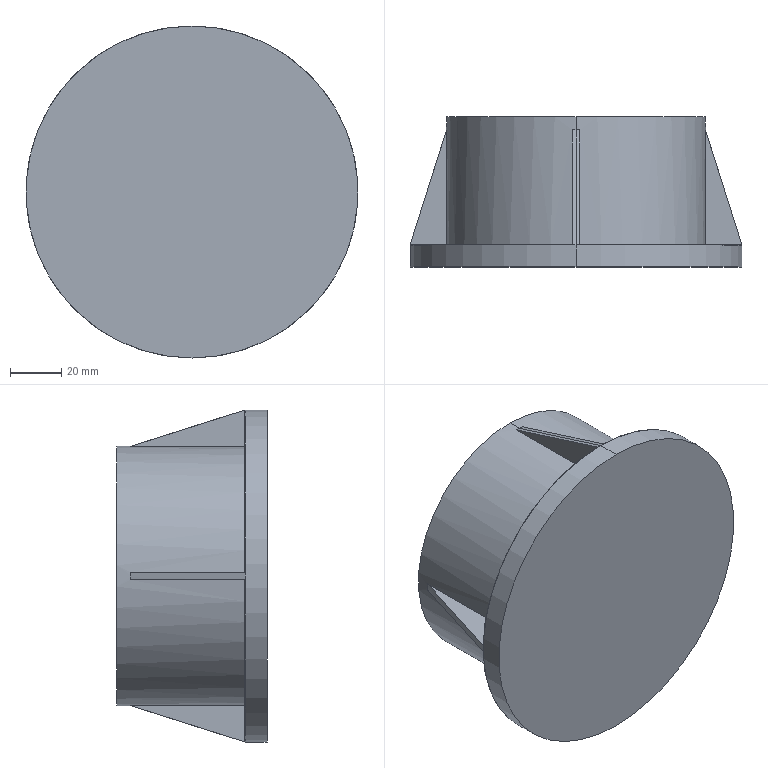Part | SolidWorks | features SavedExtBody 1 | 1 solid | 23 faces | box 129.827 x 58.73 x 129.827 mm | volume 343940 mm3 | plane 15 | cylinder 6 | cone 2 | commonest cylinder face diameters 67.426 x2 101.384 x2 129.827 x2
STEP:
#1=CARTESIAN_POINT('',(0.,-363.124,129.914));
#2=VERTEX_POINT('',#1);
#3=CARTESIAN_POINT('',(0.,-363.124,0.08649));
#4=VERTEX_POINT('',#3);
#5=CARTESIAN_POINT('',(0.,-363.124,65.));
#6=DIRECTION('',(0.,1.,0.));
#7=DIRECTION('',(0.,0.,1.));
#8=AXIS2_PLACEMENT_3D('',#5,#6,#7);
#9=CIRCLE('',#8,64.914);
#10=EDGE_CURVE('',#2,#4,#9,.T.);
#11=ORIENTED_EDGE('',*,*,#10,.T.);
#12=CARTESIAN_POINT('',(0.,-354.549,0.08649));
#13=VERTEX_POINT('',#12);
#14=CARTESIAN_POINT('',(0.,-204.512,0.08649));
#15=DIRECTION('',(0.,1.,0.));
#16=VECTOR('',#15,1000.);
#17=LINE('',#14,#16);
#18=EDGE_CURVE('',#4,#13,#17,.T.);
#19=ORIENTED_EDGE('',*,*,#18,.T.);
#20=CARTESIAN_POINT('',(0.,-354.549,129.914));
#21=VERTEX_POINT('',#20);
#22=CARTESIAN_POINT('',(0.,-354.549,65.));
#23=DIRECTION('',(0.,1.,0.));
#24=DIRECTION('',(0.,0.,1.));
#25=AXIS2_PLACEMENT_3D('',#22,#23,#24);
#26=CIRCLE('',#25,64.914);
#27=EDGE_CURVE('',#21,#13,#26,.T.);
#28=ORIENTED_EDGE('',*,*,#27,.F.);
#29=CARTESIAN_POINT('',(0.,-204.512,129.914));
#30=DIRECTION('',(0.,1.,0.));
#31=VECTOR('',#30,1000.);
#32=LINE('',#29,#31);
#33=EDGE_CURVE('',#2,#21,#32,.T.);
#34=ORIENTED_EDGE('',*,*,#33,.F.);
#35=EDGE_LOOP('',(#11,#19,#28,#34));
#36=FACE_OUTER_BOUND('',#35,.T.);
#37=CARTESIAN_POINT('',(0.,-204.512,65.));
#38=DIRECTION('',(0.,1.,0.));
#39=DIRECTION('',(0.,0.,1.));
#40=AXIS2_PLACEMENT_3D('',#37,#38,#39);
#41=CYLINDRICAL_SURFACE('',#40,64.914);
#42=ADVANCED_FACE('',(#36),#41,.T.);
#43=CARTESIAN_POINT('',(0.,-309.594,115.692));
#44=VERTEX_POINT('',#43);
#45=CARTESIAN_POINT('',(1.5,-309.594,115.67));
#46=VERTEX_POINT('',#45);
#47=CARTESIAN_POINT('',(0.,-309.594,65.));
#48=DIRECTION('',(0.,1.,0.));
#49=DIRECTION('',(0.,0.,1.));
#50=AXIS2_PLACEMENT_3D('',#47,#48,#49);
#51=CIRCLE('',#50,50.692);
#52=EDGE_CURVE('',#44,#46,#51,.T.);
#53=ORIENTED_EDGE('',*,*,#52,.F.);
#54=CARTESIAN_POINT('',(0.,-309.594,115.692));
#55=DIRECTION('',(0.,-0.9534,0.3016));
#56=VECTOR('',#55,1000.);
#57=LINE('',#54,#56);
#58=EDGE_CURVE('',#44,#21,#57,.T.);
#59=ORIENTED_EDGE('',*,*,#58,.T.);
#60=ORIENTED_EDGE('',*,*,#27,.T.);
#61=CARTESIAN_POINT('',(0.,-309.594,14.308));
#62=VERTEX_POINT('',#61);
#63=CARTESIAN_POINT('',(0.,-309.594,14.308));
#64=DIRECTION('',(0.,-0.9534,-0.3016));
#65=VECTOR('',#64,1000.);
#66=LINE('',#63,#65);
#67=EDGE_CURVE('',#62,#13,#66,.T.);
#68=ORIENTED_EDGE('',*,*,#67,.F.);
#69=CARTESIAN_POINT('',(1.5,-309.594,14.33));
#70=VERTEX_POINT('',#69);
#71=CARTESIAN_POINT('',(0.,-309.594,65.));
#72=DIRECTION('',(0.,1.,0.));
#73=DIRECTION('',(0.,0.,1.));
#74=AXIS2_PLACEMENT_3D('',#71,#72,#73);
#75=CIRCLE('',#74,50.692);
#76=EDGE_CURVE('',#70,#62,#75,.T.);
#77=ORIENTED_EDGE('',*,*,#76,.F.);
#78=CARTESIAN_POINT('',(1.5,-354.394,0.1528));
#79=VERTEX_POINT('',#78);
#80=CARTESIAN_POINT('',(1.5,-354.394,0.1528));
#81=CARTESIAN_POINT('',(1.5,-339.461,4.878));
#82=CARTESIAN_POINT('',(1.5,-324.527,9.604));
#83=CARTESIAN_POINT('',(1.5,-309.594,14.33));
#84=B_SPLINE_CURVE_WITH_KNOTS('',3,(#80,#81,#82,#83),.UNSPECIFIED.,.F.,.F.,(4,4),(0.0493,0.09629),.UNSPECIFIED.);
#85=EDGE_CURVE('',#79,#70,#84,.T.);
#86=ORIENTED_EDGE('',*,*,#85,.F.);
#87=CARTESIAN_POINT('',(64.847,-354.394,63.5));
#88=VERTEX_POINT('',#87);
#89=CARTESIAN_POINT('',(0.,-354.394,65.));
#90=DIRECTION('',(0.,-1.,0.));
#91=DIRECTION('',(-1.,0.,0.));
#92=AXIS2_PLACEMENT_3D('',#89,#90,#91);
#93=CIRCLE('',#92,64.865);
#94=EDGE_CURVE('',#79,#88,#93,.T.);
#95=ORIENTED_EDGE('',*,*,#94,.T.);
#96=CARTESIAN_POINT('',(50.67,-309.594,63.5));
#97=VERTEX_POINT('',#96);
#98=CARTESIAN_POINT('',(50.67,-309.594,63.5));
#99=CARTESIAN_POINT('',(51.247,-311.417,63.5));
#100=CARTESIAN_POINT('',(51.824,-313.241,63.5));
#101=CARTESIAN_POINT('',(52.402,-315.065,63.5));
#102=CARTESIAN_POINT('',(56.55,-328.175,63.5));
#103=CARTESIAN_POINT('',(60.699,-341.285,63.5));
#104=CARTESIAN_POINT('',(64.847,-354.394,63.5));
#105=B_SPLINE_CURVE_WITH_KNOTS('',3,(#98,#99,#100,#101,#102,#103,#104),.UNSPECIFIED.,.F.,.F.,(4,3,4),(0.0493,0.05504,0.09629),.UNSPECIFIED.);
#106=EDGE_CURVE('',#97,#88,#105,.T.);
#107=ORIENTED_EDGE('',*,*,#106,.F.);
#108=CARTESIAN_POINT('',(50.67,-309.594,66.5));
#109=VERTEX_POINT('',#108);
#110=CARTESIAN_POINT('',(0.,-309.594,65.));
#111=DIRECTION('',(0.,1.,0.));
#112=DIRECTION('',(0.,0.,1.));
#113=AXIS2_PLACEMENT_3D('',#110,#111,#112);
#114=CIRCLE('',#113,50.692);
#115=EDGE_CURVE('',#109,#97,#114,.T.);
#116=ORIENTED_EDGE('',*,*,#115,.F.);
#117=CARTESIAN_POINT('',(64.847,-354.394,66.5));
#118=VERTEX_POINT('',#117);
#119=CARTESIAN_POINT('',(64.847,-354.394,66.5));
#120=CARTESIAN_POINT('',(60.122,-339.461,66.5));
#121=CARTESIAN_POINT('',(55.396,-324.527,66.5));
#122=CARTESIAN_POINT('',(50.67,-309.594,66.5));
#123=B_SPLINE_CURVE_WITH_KNOTS('',3,(#119,#120,#121,#122),.UNSPECIFIED.,.F.,.F.,(4,4),(0.0493,0.09629),.UNSPECIFIED.);
#124=EDGE_CURVE('',#118,#109,#123,.T.);
#125=ORIENTED_EDGE('',*,*,#124,.F.);
#126=CARTESIAN_POINT('',(1.5,-354.394,129.847));
#127=VERTEX_POINT('',#126);
#128=CARTESIAN_POINT('',(0.,-354.394,65.));
#129=DIRECTION('',(0.,-1.,0.));
#130=DIRECTION('',(0.,0.,-1.));
#131=AXIS2_PLACEMENT_3D('',#128,#129,#130);
#132=CIRCLE('',#131,64.865);
#133=EDGE_CURVE('',#118,#127,#132,.T.);
#134=ORIENTED_EDGE('',*,*,#133,.T.);
#135=CARTESIAN_POINT('',(1.5,-309.594,115.67));
#136=CARTESIAN_POINT('',(1.5,-311.417,116.247));
#137=CARTESIAN_POINT('',(1.5,-313.241,116.824));
#138=CARTESIAN_POINT('',(1.5,-315.065,117.402));
#139=CARTESIAN_POINT('',(1.5,-328.175,121.55));
#140=CARTESIAN_POINT('',(1.5,-341.285,125.699));
#141=CARTESIAN_POINT('',(1.5,-354.394,129.847));
#142=B_SPLINE_CURVE_WITH_KNOTS('',3,(#135,#136,#137,#138,#139,#140,#141),.UNSPECIFIED.,.F.,.F.,(4,3,4),(0.0493,0.05504,0.09629),.UNSPECIFIED.);
#143=EDGE_CURVE('',#46,#127,#142,.T.);
#144=ORIENTED_EDGE('',*,*,#143,.F.);
#145=EDGE_LOOP('',(#53,#59,#60,#68,#77,#86,#95,#107,#116,#125,#134,#144));
#146=FACE_OUTER_BOUND('',#145,.T.);
#147=CARTESIAN_POINT('',(0.,-309.594,65.));
#148=DIRECTION('',(0.,-1.,0.));
#149=DIRECTION('',(0.,0.,-1.));
#150=AXIS2_PLACEMENT_3D('',#147,#148,#149);
#151=CONICAL_SURFACE('',#150,50.692,0.3064);
#152=ADVANCED_FACE('',(#146),#151,.T.);
#153=ORIENTED_EDGE('',*,*,#76,.T.);
#154=CARTESIAN_POINT('',(0.,-304.394,14.308));
#155=VERTEX_POINT('',#154);
#156=CARTESIAN_POINT('',(0.,-204.512,14.308));
#157=DIRECTION('',(0.,1.,0.));
#158=VECTOR('',#157,1000.);
#159=LINE('',#156,#158);
#160=EDGE_CURVE('',#62,#155,#159,.T.);
#161=ORIENTED_EDGE('',*,*,#160,.T.);
#162=CARTESIAN_POINT('',(0.,-304.394,115.692));
#163=VERTEX_POINT('',#162);
#164=CARTESIAN_POINT('',(0.,-304.394,65.));
#165=DIRECTION('',(0.,1.,0.));
#166=DIRECTION('',(0.,0.,1.));
#167=AXIS2_PLACEMENT_3D('',#164,#165,#166);
#168=CIRCLE('',#167,50.692);
#169=EDGE_CURVE('',#163,#155,#168,.T.);
#170=ORIENTED_EDGE('',*,*,#169,.F.);
#171=CARTESIAN_POINT('',(0.,-204.512,115.692));
#172=DIRECTION('',(0.,1.,0.));
#173=VECTOR('',#172,1000.);
#174=LINE('',#171,#173);
#175=EDGE_CURVE('',#44,#163,#174,.T.);
#176=ORIENTED_EDGE('',*,*,#175,.F.);
#177=ORIENTED_EDGE('',*,*,#52,.T.);
#178=CARTESIAN_POINT('',(1.5,-354.394,115.67));
#179=VERTEX_POINT('',#178);
#180=CARTESIAN_POINT('',(1.5,-354.394,115.67));
#181=DIRECTION('',(0.,1.,0.));
#182=VECTOR('',#181,1000.);
#183=LINE('',#180,#182);
#184=EDGE_CURVE('',#179,#46,#183,.T.);
#185=ORIENTED_EDGE('',*,*,#184,.F.);
#186=CARTESIAN_POINT('',(50.67,-354.394,66.5));
#187=VERTEX_POINT('',#186);
#188=CARTESIAN_POINT('',(0.,-354.394,65.));
#189=DIRECTION('',(0.,-1.,0.));
#190=DIRECTION('',(0.,0.,-1.));
#191=AXIS2_PLACEMENT_3D('',#188,#189,#190);
#192=CIRCLE('',#191,50.692);
#193=EDGE_CURVE('',#187,#179,#192,.T.);
#194=ORIENTED_EDGE('',*,*,#193,.F.);
#195=CARTESIAN_POINT('',(50.67,-354.394,66.5));
#196=DIRECTION('',(0.,1.,0.));
#197=VECTOR('',#196,1000.);
#198=LINE('',#195,#197);
#199=EDGE_CURVE('',#187,#109,#198,.T.);
#200=ORIENTED_EDGE('',*,*,#199,.T.);
#201=ORIENTED_EDGE('',*,*,#115,.T.);
#202=CARTESIAN_POINT('',(50.67,-354.394,63.5));
#203=VERTEX_POINT('',#202);
#204=CARTESIAN_POINT('',(50.67,-354.394,63.5));
#205=DIRECTION('',(0.,1.,0.));
#206=VECTOR('',#205,1000.);
#207=LINE('',#204,#206);
#208=EDGE_CURVE('',#203,#97,#207,.T.);
#209=ORIENTED_EDGE('',*,*,#208,.F.);
#210=CARTESIAN_POINT('',(1.5,-354.394,14.33));
#211=VERTEX_POINT('',#210);
#212=CARTESIAN_POINT('',(0.,-354.394,65.));
#213=DIRECTION('',(0.,-1.,0.));
#214=DIRECTION('',(-1.,0.,0.));
#215=AXIS2_PLACEMENT_3D('',#212,#213,#214);
#216=CIRCLE('',#215,50.692);
#217=EDGE_CURVE('',#211,#203,#216,.T.);
#218=ORIENTED_EDGE('',*,*,#217,.F.);
#219=CARTESIAN_POINT('',(1.5,-354.394,14.33));
#220=DIRECTION('',(0.,1.,0.));
#221=VECTOR('',#220,1000.);
#222=LINE('',#219,#221);
#223=EDGE_CURVE('',#211,#70,#222,.T.);
#224=ORIENTED_EDGE('',*,*,#223,.T.);
#225=EDGE_LOOP('',(#153,#161,#170,#176,#177,#185,#194,#200,#201,#209,#218,#224));
#226=FACE_OUTER_BOUND('',#225,.T.);
#227=CARTESIAN_POINT('',(0.,-204.512,65.));
#228=DIRECTION('',(0.,1.,0.));
#229=DIRECTION('',(0.,0.,1.));
#230=AXIS2_PLACEMENT_3D('',#227,#228,#229);
#231=CYLINDRICAL_SURFACE('',#230,50.692);
#232=ADVANCED_FACE('',(#226),#231,.T.);
#233=CARTESIAN_POINT('',(0.,-354.549,31.287));
#234=VERTEX_POINT('',#233);
#235=CARTESIAN_POINT('',(0.,-354.549,98.713));
#236=VERTEX_POINT('',#235);
#237=CARTESIAN_POINT('',(0.,-354.549,65.));
#238=DIRECTION('',(0.,1.,0.));
#239=DIRECTION('',(0.,0.,1.));
#240=AXIS2_PLACEMENT_3D('',#237,#238,#239);
#241=CIRCLE('',#240,33.713);
#242=EDGE_CURVE('',#234,#236,#241,.T.);
#243=ORIENTED_EDGE('',*,*,#242,.F.);
#244=CARTESIAN_POINT('',(0.,-304.394,31.287));
#245=VERTEX_POINT('',#244);
#246=CARTESIAN_POINT('',(0.,-204.512,31.287));
#247=DIRECTION('',(0.,1.,0.));
#248=VECTOR('',#247,1000.);
#249=LINE('',#246,#248);
#250=EDGE_CURVE('',#234,#245,#249,.T.);
#251=ORIENTED_EDGE('',*,*,#250,.T.);
#252=CARTESIAN_POINT('',(0.,-304.394,98.713));
#253=VERTEX_POINT('',#252);
#254=CARTESIAN_POINT('',(0.,-304.394,65.));
#255=DIRECTION('',(0.,1.,0.));
#256=DIRECTION('',(0.,0.,1.));
#257=AXIS2_PLACEMENT_3D('',#254,#255,#256);
#258=CIRCLE('',#257,33.713);
#259=EDGE_CURVE('',#245,#253,#258,.T.);
#260=ORIENTED_EDGE('',*,*,#259,.T.);
#261=CARTESIAN_POINT('',(0.,-204.512,98.713));
#262=DIRECTION('',(0.,1.,0.));
#263=VECTOR('',#262,1000.);
#264=LINE('',#261,#263);
#265=EDGE_CURVE('',#236,#253,#264,.T.);
#266=ORIENTED_EDGE('',*,*,#265,.F.);
#267=EDGE_LOOP('',(#243,#251,#260,#266));
#268=FACE_OUTER_BOUND('',#267,.T.);
#269=CARTESIAN_POINT('',(0.,-204.512,65.));
#270=DIRECTION('',(0.,1.,0.));
#271=DIRECTION('',(0.,0.,1.));
#272=AXIS2_PLACEMENT_3D('',#269,#270,#271);
#273=CYLINDRICAL_SURFACE('',#272,33.713);
#274=ADVANCED_FACE('',(#268),#273,.F.);
#275=ORIENTED_EDGE('',*,*,#85,.T.);
#276=ORIENTED_EDGE('',*,*,#223,.F.);
#277=CARTESIAN_POINT('',(1.5,-354.394,0.1038));
#278=DIRECTION('',(0.,0.,1.));
#279=VECTOR('',#278,1000.);
#280=LINE('',#277,#279);
#281=EDGE_CURVE('',#79,#211,#280,.T.);
#282=ORIENTED_EDGE('',*,*,#281,.F.);
#283=EDGE_LOOP('',(#275,#276,#282));
#284=FACE_OUTER_BOUND('',#283,.T.);
#285=CARTESIAN_POINT('',(1.5,-354.394,0.1038));
#286=DIRECTION('',(-1.,0.,0.));
#287=DIRECTION('',(0.,0.,1.));
#288=AXIS2_PLACEMENT_3D('',#285,#286,#287);
#289=PLANE('',#288);
#290=ADVANCED_FACE('',(#284),#289,.F.);
#291=ORIENTED_EDGE('',*,*,#106,.T.);
#292=CARTESIAN_POINT('',(64.896,-354.394,63.5));
#293=DIRECTION('',(1.,0.,0.));
#294=VECTOR('',#293,1000.);
#295=LINE('',#292,#294);
#296=EDGE_CURVE('',#203,#88,#295,.T.);
#297=ORIENTED_EDGE('',*,*,#296,.F.);
#298=ORIENTED_EDGE('',*,*,#208,.T.);
#299=EDGE_LOOP('',(#291,#297,#298));
#300=FACE_OUTER_BOUND('',#299,.T.);
#301=CARTESIAN_POINT('',(64.896,-354.394,63.5));
#302=DIRECTION('',(0.,0.,1.));
#303=DIRECTION('',(1.,0.,0.));
#304=AXIS2_PLACEMENT_3D('',#301,#302,#303);
#305=PLANE('',#304);
#306=ADVANCED_FACE('',(#300),#305,.F.);
#307=ORIENTED_EDGE('',*,*,#281,.T.);
#308=ORIENTED_EDGE('',*,*,#217,.T.);
#309=ORIENTED_EDGE('',*,*,#296,.T.);
#310=ORIENTED_EDGE('',*,*,#94,.F.);
#311=EDGE_LOOP('',(#307,#308,#309,#310));
#312=FACE_OUTER_BOUND('',#311,.T.);
#313=CARTESIAN_POINT('',(0.,-354.394,65.));
#314=DIRECTION('',(0.,1.,0.));
#315=DIRECTION('',(-1.,0.,0.));
#316=AXIS2_PLACEMENT_3D('',#313,#314,#315);
#317=PLANE('',#316);
#318=ADVANCED_FACE('',(#312),#317,.T.);
#319=ORIENTED_EDGE('',*,*,#124,.T.);
#320=ORIENTED_EDGE('',*,*,#199,.F.);
#321=CARTESIAN_POINT('',(64.896,-354.394,66.5));
#322=DIRECTION('',(-1.,0.,0.));
#323=VECTOR('',#322,1000.);
#324=LINE('',#321,#323);
#325=EDGE_CURVE('',#118,#187,#324,.T.);
#326=ORIENTED_EDGE('',*,*,#325,.F.);
#327=EDGE_LOOP('',(#319,#320,#326));
#328=FACE_OUTER_BOUND('',#327,.T.);
#329=CARTESIAN_POINT('',(64.896,-354.394,66.5));
#330=DIRECTION('',(0.,0.,-1.));
#331=DIRECTION('',(-1.,0.,0.));
#332=AXIS2_PLACEMENT_3D('',#329,#330,#331);
#333=PLANE('',#332);
#334=ADVANCED_FACE('',(#328),#333,.F.);
#335=ORIENTED_EDGE('',*,*,#143,.T.);
#336=CARTESIAN_POINT('',(1.5,-354.394,129.896));
#337=DIRECTION('',(0.,0.,1.));
#338=VECTOR('',#337,1000.);
#339=LINE('',#336,#338);
#340=EDGE_CURVE('',#179,#127,#339,.T.);
#341=ORIENTED_EDGE('',*,*,#340,.F.);
#342=ORIENTED_EDGE('',*,*,#184,.T.);
#343=EDGE_LOOP('',(#335,#341,#342));
#344=FACE_OUTER_BOUND('',#343,.T.);
#345=CARTESIAN_POINT('',(1.5,-354.394,129.896));
#346=DIRECTION('',(-1.,0.,0.));
#347=DIRECTION('',(0.,0.,1.));
#348=AXIS2_PLACEMENT_3D('',#345,#346,#347);
#349=PLANE('',#348);
#350=ADVANCED_FACE('',(#344),#349,.F.);
#351=ORIENTED_EDGE('',*,*,#325,.T.);
#352=ORIENTED_EDGE('',*,*,#193,.T.);
#353=ORIENTED_EDGE('',*,*,#340,.T.);
#354=ORIENTED_EDGE('',*,*,#133,.F.);
#355=EDGE_LOOP('',(#351,#352,#353,#354));
#356=FACE_OUTER_BOUND('',#355,.T.);
#357=CARTESIAN_POINT('',(0.,-354.394,65.));
#358=DIRECTION('',(0.,1.,0.));
#359=DIRECTION('',(0.,0.,-1.));
#360=AXIS2_PLACEMENT_3D('',#357,#358,#359);
#361=PLANE('',#360);
#362=ADVANCED_FACE('',(#356),#361,.T.);
#363=CARTESIAN_POINT('',(-1.5,-354.394,129.847));
#364=VERTEX_POINT('',#363);
#365=CARTESIAN_POINT('',(-1.5,-309.594,115.67));
#366=VERTEX_POINT('',#365);
#367=CARTESIAN_POINT('',(-1.5,-354.394,129.847));
#368=CARTESIAN_POINT('',(-1.5,-339.461,125.122));
#369=CARTESIAN_POINT('',(-1.5,-324.527,120.396));
#370=CARTESIAN_POINT('',(-1.5,-309.594,115.67));
#371=B_SPLINE_CURVE_WITH_KNOTS('',3,(#367,#368,#369,#370),.UNSPECIFIED.,.F.,.F.,(4,4),(0.0493,0.09629),.UNSPECIFIED.);
#372=EDGE_CURVE('',#364,#366,#371,.T.);
#373=ORIENTED_EDGE('',*,*,#372,.T.);
#374=CARTESIAN_POINT('',(-1.5,-354.394,115.67));
#375=VERTEX_POINT('',#374);
#376=CARTESIAN_POINT('',(-1.5,-354.394,115.67));
#377=DIRECTION('',(0.,1.,0.));
#378=VECTOR('',#377,1000.);
#379=LINE('',#376,#378);
#380=EDGE_CURVE('',#375,#366,#379,.T.);
#381=ORIENTED_EDGE('',*,*,#380,.F.);
#382=CARTESIAN_POINT('',(-1.5,-354.394,129.896));
#383=DIRECTION('',(0.,0.,-1.));
#384=VECTOR('',#383,1000.);
#385=LINE('',#382,#384);
#386=EDGE_CURVE('',#364,#375,#385,.T.);
#387=ORIENTED_EDGE('',*,*,#386,.F.);
#388=EDGE_LOOP('',(#373,#381,#387));
#389=FACE_OUTER_BOUND('',#388,.T.);
#390=CARTESIAN_POINT('',(-1.5,-354.394,129.896));
#391=DIRECTION('',(1.,0.,0.));
#392=DIRECTION('',(0.,0.,-1.));
#393=AXIS2_PLACEMENT_3D('',#390,#391,#392);
#394=PLANE('',#393);
#395=ADVANCED_FACE('',(#389),#394,.F.);
#396=CARTESIAN_POINT('',(-50.67,-309.594,66.5));
#397=VERTEX_POINT('',#396);
#398=CARTESIAN_POINT('',(-64.847,-354.394,66.5));
#399=VERTEX_POINT('',#398);
#400=CARTESIAN_POINT('',(-50.67,-309.594,66.5));
#401=CARTESIAN_POINT('',(-51.247,-311.417,66.5));
#402=CARTESIAN_POINT('',(-51.824,-313.241,66.5));
#403=CARTESIAN_POINT('',(-52.402,-315.065,66.5));
#404=CARTESIAN_POINT('',(-56.55,-328.175,66.5));
#405=CARTESIAN_POINT('',(-60.699,-341.285,66.5));
#406=CARTESIAN_POINT('',(-64.847,-354.394,66.5));
#407=B_SPLINE_CURVE_WITH_KNOTS('',3,(#400,#401,#402,#403,#404,#405,#406),.UNSPECIFIED.,.F.,.F.,(4,3,4),(0.0493,0.05504,0.09629),.UNSPECIFIED.);
#408=EDGE_CURVE('',#397,#399,#407,.T.);
#409=ORIENTED_EDGE('',*,*,#408,.T.);
#410=CARTESIAN_POINT('',(-50.67,-354.394,66.5));
#411=VERTEX_POINT('',#410);
#412=CARTESIAN_POINT('',(-64.896,-354.394,66.5));
#413=DIRECTION('',(-1.,0.,0.));
#414=VECTOR('',#413,1000.);
#415=LINE('',#412,#414);
#416=EDGE_CURVE('',#411,#399,#415,.T.);
#417=ORIENTED_EDGE('',*,*,#416,.F.);
#418=CARTESIAN_POINT('',(-50.67,-354.394,66.5));
#419=DIRECTION('',(0.,1.,0.));
#420=VECTOR('',#419,1000.);
#421=LINE('',#418,#420);
#422=EDGE_CURVE('',#411,#397,#421,.T.);
#423=ORIENTED_EDGE('',*,*,#422,.T.);
#424=EDGE_LOOP('',(#409,#417,#423));
#425=FACE_OUTER_BOUND('',#424,.T.);
#426=CARTESIAN_POINT('',(-64.896,-354.394,66.5));
#427=DIRECTION('',(0.,0.,-1.));
#428=DIRECTION('',(-1.,0.,0.));
#429=AXIS2_PLACEMENT_3D('',#426,#427,#428);
#430=PLANE('',#429);
#431=ADVANCED_FACE('',(#425),#430,.F.);
#432=ORIENTED_EDGE('',*,*,#386,.T.);
#433=CARTESIAN_POINT('',(0.,-354.394,65.));
#434=DIRECTION('',(0.,-1.,0.));
#435=DIRECTION('',(1.,0.,0.));
#436=AXIS2_PLACEMENT_3D('',#433,#434,#435);
#437=CIRCLE('',#436,50.692);
#438=EDGE_CURVE('',#375,#411,#437,.T.);
#439=ORIENTED_EDGE('',*,*,#438,.T.);
#440=ORIENTED_EDGE('',*,*,#416,.T.);
#441=CARTESIAN_POINT('',(0.,-354.394,65.));
#442=DIRECTION('',(0.,-1.,0.));
#443=DIRECTION('',(1.,0.,0.));
#444=AXIS2_PLACEMENT_3D('',#441,#442,#443);
#445=CIRCLE('',#444,64.865);
#446=EDGE_CURVE('',#364,#399,#445,.T.);
#447=ORIENTED_EDGE('',*,*,#446,.F.);
#448=EDGE_LOOP('',(#432,#439,#440,#447));
#449=FACE_OUTER_BOUND('',#448,.T.);
#450=CARTESIAN_POINT('',(0.,-354.394,65.));
#451=DIRECTION('',(0.,1.,0.));
#452=DIRECTION('',(1.,0.,0.));
#453=AXIS2_PLACEMENT_3D('',#450,#451,#452);
#454=PLANE('',#453);
#455=ADVANCED_FACE('',(#449),#454,.T.);
#456=ORIENTED_EDGE('',*,*,#250,.F.);
#457=CARTESIAN_POINT('',(0.,-354.549,65.));
#458=DIRECTION('',(0.,1.,0.));
#459=DIRECTION('',(0.,0.,1.));
#460=AXIS2_PLACEMENT_3D('',#457,#458,#459);
#461=CIRCLE('',#460,33.713);
#462=EDGE_CURVE('',#236,#234,#461,.T.);
#463=ORIENTED_EDGE('',*,*,#462,.F.);
#464=ORIENTED_EDGE('',*,*,#265,.T.);
#465=CARTESIAN_POINT('',(0.,-304.394,65.));
#466=DIRECTION('',(0.,1.,0.));
#467=DIRECTION('',(0.,0.,1.));
#468=AXIS2_PLACEMENT_3D('',#465,#466,#467);
#469=CIRCLE('',#468,33.713);
#470=EDGE_CURVE('',#253,#245,#469,.T.);
#471=ORIENTED_EDGE('',*,*,#470,.T.);
#472=EDGE_LOOP('',(#456,#463,#464,#471));
#473=FACE_OUTER_BOUND('',#472,.T.);
#474=CARTESIAN_POINT('',(0.,-204.512,65.));
#475=DIRECTION('',(0.,1.,0.));
#476=DIRECTION('',(0.,0.,1.));
#477=AXIS2_PLACEMENT_3D('',#474,#475,#476);
#478=CYLINDRICAL_SURFACE('',#477,33.713);
#479=ADVANCED_FACE('',(#473),#478,.F.);
#480=ORIENTED_EDGE('',*,*,#169,.T.);
#481=CARTESIAN_POINT('',(0.,-304.394,65.));
#482=DIRECTION('',(0.,1.,0.));
#483=DIRECTION('',(0.,0.,1.));
#484=AXIS2_PLACEMENT_3D('',#481,#482,#483);
#485=CIRCLE('',#484,50.692);
#486=EDGE_CURVE('',#155,#163,#485,.T.);
#487=ORIENTED_EDGE('',*,*,#486,.T.);
#488=EDGE_LOOP('',(#480,#487));
#489=FACE_OUTER_BOUND('',#488,.T.);
#490=ORIENTED_EDGE('',*,*,#470,.F.);
#491=ORIENTED_EDGE('',*,*,#259,.F.);
#492=EDGE_LOOP('',(#490,#491));
#493=FACE_BOUND('',#492,.T.);
#494=CARTESIAN_POINT('',(-33.713,-304.394,65.));
#495=DIRECTION('',(0.,1.,0.));
#496=DIRECTION('',(0.,0.,1.));
#497=AXIS2_PLACEMENT_3D('',#494,#495,#496);
#498=PLANE('',#497);
#499=ADVANCED_FACE('',(#489,#493),#498,.T.);
#500=ORIENTED_EDGE('',*,*,#160,.F.);
#501=CARTESIAN_POINT('',(-1.5,-309.594,14.33));
#502=VERTEX_POINT('',#501);
#503=CARTESIAN_POINT('',(0.,-309.594,65.));
#504=DIRECTION('',(0.,1.,0.));
#505=DIRECTION('',(0.,0.,1.));
#506=AXIS2_PLACEMENT_3D('',#503,#504,#505);
#507=CIRCLE('',#506,50.692);
#508=EDGE_CURVE('',#62,#502,#507,.T.);
#509=ORIENTED_EDGE('',*,*,#508,.T.);
#510=CARTESIAN_POINT('',(-1.5,-354.394,14.33));
#511=VERTEX_POINT('',#510);
#512=CARTESIAN_POINT('',(-1.5,-354.394,14.33));
#513=DIRECTION('',(0.,1.,0.));
#514=VECTOR('',#513,1000.);
#515=LINE('',#512,#514);
#516=EDGE_CURVE('',#511,#502,#515,.T.);
#517=ORIENTED_EDGE('',*,*,#516,.F.);
#518=CARTESIAN_POINT('',(-50.67,-354.394,63.5));
#519=VERTEX_POINT('',#518);
#520=CARTESIAN_POINT('',(0.,-354.394,65.));
#521=DIRECTION('',(0.,-1.,0.));
#522=DIRECTION('',(0.,0.,1.));
#523=AXIS2_PLACEMENT_3D('',#520,#521,#522);
#524=CIRCLE('',#523,50.692);
#525=EDGE_CURVE('',#519,#511,#524,.T.);
#526=ORIENTED_EDGE('',*,*,#525,.F.);
#527=CARTESIAN_POINT('',(-50.67,-309.594,63.5));
#528=VERTEX_POINT('',#527);
#529=CARTESIAN_POINT('',(-50.67,-354.394,63.5));
#530=DIRECTION('',(0.,1.,0.));
#531=VECTOR('',#530,1000.);
#532=LINE('',#529,#531);
#533=EDGE_CURVE('',#519,#528,#532,.T.);
#534=ORIENTED_EDGE('',*,*,#533,.T.);
#535=CARTESIAN_POINT('',(0.,-309.594,65.));
#536=DIRECTION('',(0.,1.,0.));
#537=DIRECTION('',(0.,0.,1.));
#538=AXIS2_PLACEMENT_3D('',#535,#536,#537);
#539=CIRCLE('',#538,50.692);
#540=EDGE_CURVE('',#528,#397,#539,.T.);
#541=ORIENTED_EDGE('',*,*,#540,.T.);
#542=ORIENTED_EDGE('',*,*,#422,.F.);
#543=ORIENTED_EDGE('',*,*,#438,.F.);
#544=ORIENTED_EDGE('',*,*,#380,.T.);
#545=CARTESIAN_POINT('',(0.,-309.594,65.));
#546=DIRECTION('',(0.,1.,0.));
#547=DIRECTION('',(0.,0.,1.));
#548=AXIS2_PLACEMENT_3D('',#545,#546,#547);
#549=CIRCLE('',#548,50.692);
#550=EDGE_CURVE('',#366,#44,#549,.T.);
#551=ORIENTED_EDGE('',*,*,#550,.T.);
#552=ORIENTED_EDGE('',*,*,#175,.T.);
#553=ORIENTED_EDGE('',*,*,#486,.F.);
#554=EDGE_LOOP('',(#500,#509,#517,#526,#534,#541,#542,#543,#544,#551,#552,#553));
#555=FACE_OUTER_BOUND('',#554,.T.);
#556=CARTESIAN_POINT('',(0.,-204.512,65.));
#557=DIRECTION('',(0.,1.,0.));
#558=DIRECTION('',(0.,0.,1.));
#559=AXIS2_PLACEMENT_3D('',#556,#557,#558);
#560=CYLINDRICAL_SURFACE('',#559,50.692);
#561=ADVANCED_FACE('',(#555),#560,.T.);
#562=ORIENTED_EDGE('',*,*,#58,.F.);
#563=ORIENTED_EDGE('',*,*,#550,.F.);
#564=ORIENTED_EDGE('',*,*,#372,.F.);
#565=ORIENTED_EDGE('',*,*,#446,.T.);
#566=ORIENTED_EDGE('',*,*,#408,.F.);
#567=ORIENTED_EDGE('',*,*,#540,.F.);
#568=CARTESIAN_POINT('',(-64.847,-354.394,63.5));
#569=VERTEX_POINT('',#568);
#570=CARTESIAN_POINT('',(-64.847,-354.394,63.5));
#571=CARTESIAN_POINT('',(-60.122,-339.461,63.5));
#572=CARTESIAN_POINT('',(-55.396,-324.527,63.5));
#573=CARTESIAN_POINT('',(-50.67,-309.594,63.5));
#574=B_SPLINE_CURVE_WITH_KNOTS('',3,(#570,#571,#572,#573),.UNSPECIFIED.,.F.,.F.,(4,4),(0.0493,0.09629),.UNSPECIFIED.);
#575=EDGE_CURVE('',#569,#528,#574,.T.);
#576=ORIENTED_EDGE('',*,*,#575,.F.);
#577=CARTESIAN_POINT('',(-1.5,-354.394,0.1528));
#578=VERTEX_POINT('',#577);
#579=CARTESIAN_POINT('',(0.,-354.394,65.));
#580=DIRECTION('',(0.,-1.,0.));
#581=DIRECTION('',(0.,0.,1.));
#582=AXIS2_PLACEMENT_3D('',#579,#580,#581);
#583=CIRCLE('',#582,64.865);
#584=EDGE_CURVE('',#569,#578,#583,.T.);
#585=ORIENTED_EDGE('',*,*,#584,.T.);
#586=CARTESIAN_POINT('',(-1.5,-309.594,14.33));
#587=CARTESIAN_POINT('',(-1.5,-311.417,13.753));
#588=CARTESIAN_POINT('',(-1.5,-313.241,13.176));
#589=CARTESIAN_POINT('',(-1.5,-315.065,12.598));
#590=CARTESIAN_POINT('',(-1.5,-328.175,8.45));
#591=CARTESIAN_POINT('',(-1.5,-341.285,4.301));
#592=CARTESIAN_POINT('',(-1.5,-354.394,0.1528));
#593=B_SPLINE_CURVE_WITH_KNOTS('',3,(#586,#587,#588,#589,#590,#591,#592),.UNSPECIFIED.,.F.,.F.,(4,3,4),(0.0493,0.05504,0.09629),.UNSPECIFIED.);
#594=EDGE_CURVE('',#502,#578,#593,.T.);
#595=ORIENTED_EDGE('',*,*,#594,.F.);
#596=ORIENTED_EDGE('',*,*,#508,.F.);
#597=ORIENTED_EDGE('',*,*,#67,.T.);
#598=CARTESIAN_POINT('',(0.,-354.549,65.));
#599=DIRECTION('',(0.,1.,0.));
#600=DIRECTION('',(0.,0.,1.));
#601=AXIS2_PLACEMENT_3D('',#598,#599,#600);
#602=CIRCLE('',#601,64.914);
#603=EDGE_CURVE('',#13,#21,#602,.T.);
#604=ORIENTED_EDGE('',*,*,#603,.T.);
#605=EDGE_LOOP('',(#562,#563,#564,#565,#566,#567,#576,#585,#595,#596,#597,#604));
#606=FACE_OUTER_BOUND('',#605,.T.);
#607=CARTESIAN_POINT('',(0.,-309.594,65.));
#608=DIRECTION('',(0.,-1.,0.));
#609=DIRECTION('',(0.,0.,-1.));
#610=AXIS2_PLACEMENT_3D('',#607,#608,#609);
#611=CONICAL_SURFACE('',#610,50.692,0.3064);
#612=ADVANCED_FACE('',(#606),#611,.T.);
#613=ORIENTED_EDGE('',*,*,#18,.F.);
#614=CARTESIAN_POINT('',(0.,-363.124,65.));
#615=DIRECTION('',(0.,1.,0.));
#616=DIRECTION('',(0.,0.,1.));
#617=AXIS2_PLACEMENT_3D('',#614,#615,#616);
#618=CIRCLE('',#617,64.914);
#619=EDGE_CURVE('',#4,#2,#618,.T.);
#620=ORIENTED_EDGE('',*,*,#619,.T.);
#621=ORIENTED_EDGE('',*,*,#33,.T.);
#622=ORIENTED_EDGE('',*,*,#603,.F.);
#623=EDGE_LOOP('',(#613,#620,#621,#622));
#624=FACE_OUTER_BOUND('',#623,.T.);
#625=CARTESIAN_POINT('',(0.,-204.512,65.));
#626=DIRECTION('',(0.,1.,0.));
#627=DIRECTION('',(0.,0.,1.));
#628=AXIS2_PLACEMENT_3D('',#625,#626,#627);
#629=CYLINDRICAL_SURFACE('',#628,64.914);
#630=ADVANCED_FACE('',(#624),#629,.T.);
#631=ORIENTED_EDGE('',*,*,#10,.F.);
#632=ORIENTED_EDGE('',*,*,#619,.F.);
#633=EDGE_LOOP('',(#631,#632));
#634=FACE_OUTER_BOUND('',#633,.T.);
#635=CARTESIAN_POINT('',(-64.914,-363.124,65.));
#636=DIRECTION('',(0.,-1.,0.));
#637=DIRECTION('',(0.,0.,-1.));
#638=AXIS2_PLACEMENT_3D('',#635,#636,#637);
#639=PLANE('',#638);
#640=ADVANCED_FACE('',(#634),#639,.T.);
#641=ORIENTED_EDGE('',*,*,#462,.T.);
#642=ORIENTED_EDGE('',*,*,#242,.T.);
#643=EDGE_LOOP('',(#641,#642));
#644=FACE_OUTER_BOUND('',#643,.T.);
#645=CARTESIAN_POINT('',(-33.713,-354.549,65.));
#646=DIRECTION('',(0.,1.,0.));
#647=DIRECTION('',(0.,0.,1.));
#648=AXIS2_PLACEMENT_3D('',#645,#646,#647);
#649=PLANE('',#648);
#650=ADVANCED_FACE('',(#644),#649,.T.);
#651=ORIENTED_EDGE('',*,*,#575,.T.);
#652=ORIENTED_EDGE('',*,*,#533,.F.);
#653=CARTESIAN_POINT('',(-64.896,-354.394,63.5));
#654=DIRECTION('',(1.,0.,0.));
#655=VECTOR('',#654,1000.);
#656=LINE('',#653,#655);
#657=EDGE_CURVE('',#569,#519,#656,.T.);
#658=ORIENTED_EDGE('',*,*,#657,.F.);
#659=EDGE_LOOP('',(#651,#652,#658));
#660=FACE_OUTER_BOUND('',#659,.T.);
#661=CARTESIAN_POINT('',(-64.896,-354.394,63.5));
#662=DIRECTION('',(0.,0.,1.));
#663=DIRECTION('',(1.,0.,0.));
#664=AXIS2_PLACEMENT_3D('',#661,#662,#663);
#665=PLANE('',#664);
#666=ADVANCED_FACE('',(#660),#665,.F.);
#667=ORIENTED_EDGE('',*,*,#594,.T.);
#668=CARTESIAN_POINT('',(-1.5,-354.394,0.1038));
#669=DIRECTION('',(0.,0.,-1.));
#670=VECTOR('',#669,1000.);
#671=LINE('',#668,#670);
#672=EDGE_CURVE('',#511,#578,#671,.T.);
#673=ORIENTED_EDGE('',*,*,#672,.F.);
#674=ORIENTED_EDGE('',*,*,#516,.T.);
#675=EDGE_LOOP('',(#667,#673,#674));
#676=FACE_OUTER_BOUND('',#675,.T.);
#677=CARTESIAN_POINT('',(-1.5,-354.394,0.1038));
#678=DIRECTION('',(1.,0.,0.));
#679=DIRECTION('',(0.,0.,-1.));
#680=AXIS2_PLACEMENT_3D('',#677,#678,#679);
#681=PLANE('',#680);
#682=ADVANCED_FACE('',(#676),#681,.F.);
#683=ORIENTED_EDGE('',*,*,#657,.T.);
#684=ORIENTED_EDGE('',*,*,#525,.T.);
#685=ORIENTED_EDGE('',*,*,#672,.T.);
#686=ORIENTED_EDGE('',*,*,#584,.F.);
#687=EDGE_LOOP('',(#683,#684,#685,#686));
#688=FACE_OUTER_BOUND('',#687,.T.);
#689=CARTESIAN_POINT('',(0.,-354.394,65.));
#690=DIRECTION('',(0.,1.,0.));
#691=DIRECTION('',(0.,0.,1.));
#692=AXIS2_PLACEMENT_3D('',#689,#690,#691);
#693=PLANE('',#692);
#694=ADVANCED_FACE('',(#688),#693,.T.);
#695=CLOSED_SHELL('',(#42,#152,#232,#274,#290,#306,#318,#334,#350,#362,#395,#431,#455,#479,#499,#561,#612,#630,#640,#650,#666,#682,#694));
#696=MANIFOLD_SOLID_BREP('',#695);
#697=CARTESIAN_POINT('',(0.,0.,0.));
#698=DIRECTION('',(0.,0.,1.));
#699=DIRECTION('',(1.,0.,0.));
#700=AXIS2_PLACEMENT_3D('',#697,#698,#699);
#701=(LENGTH_UNIT()NAMED_UNIT(*)SI_UNIT(.MILLI.,.METRE.));
#702=UNCERTAINTY_MEASURE_WITH_UNIT(LENGTH_MEASURE(0.00001),#701,'','');
#703=(NAMED_UNIT(*)PLANE_ANGLE_UNIT()SI_UNIT($,.RADIAN.));
#704=(NAMED_UNIT(*)SI_UNIT($,.STERADIAN.)SOLID_ANGLE_UNIT());
#705=(GEOMETRIC_REPRESENTATION_CONTEXT(3)GLOBAL_UNCERTAINTY_ASSIGNED_CONTEXT((#702))GLOBAL_UNIT_ASSIGNED_CONTEXT((#701,#703,#704))REPRESENTATION_CONTEXT('',''));
#706=ADVANCED_BREP_SHAPE_REPRESENTATION('',(#696,#700),#705);